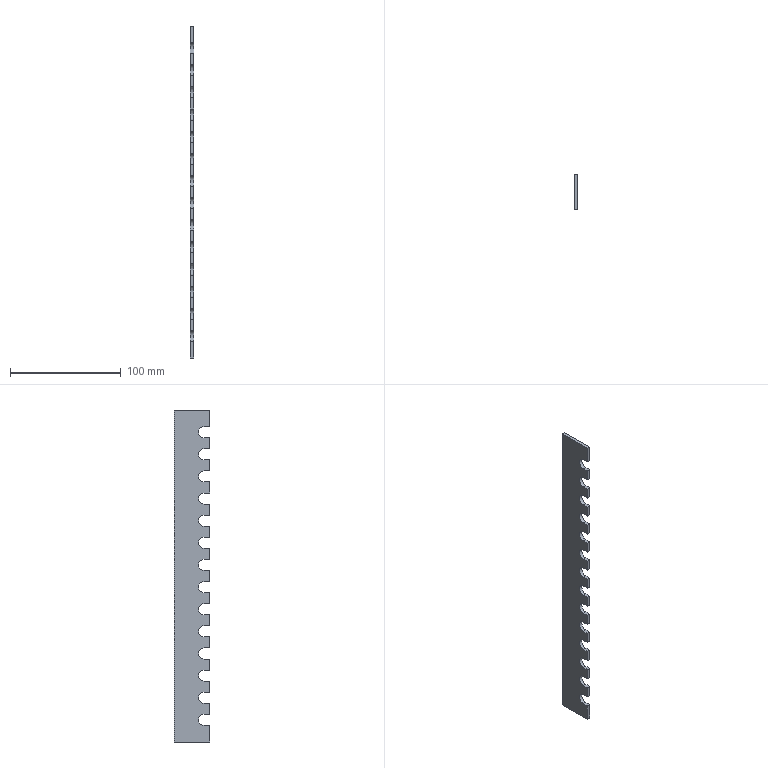Part | SolidWorks | features ExtruThin 1, ICE 1, LPattern 1 | 1 solid | 62 faces | box 3 x 32 x 300 mm | volume 25051 mm3 | plane 48 | cylinder 14 | commonest cylinder face diameters 10 x14